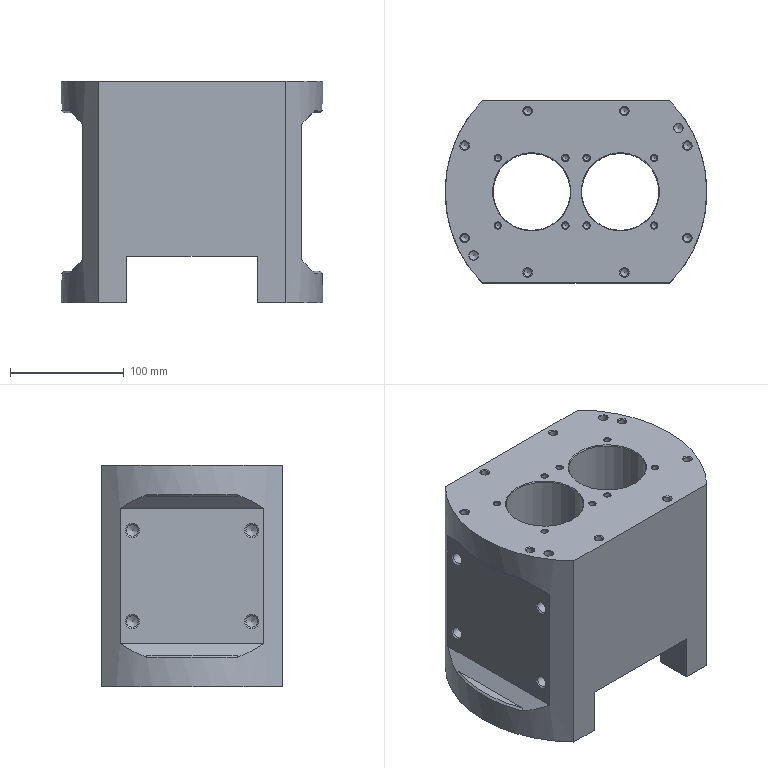NC program | NX | posted with a generic post | part box 230 x 160 x 195 mm
Lines 2916 to 3764 of 6533:
(ZLEVEL_PROFILE_COPY_1 , TOOL : D6R0.5)
N5818 T05 M6
N5820 G54
N5822 G17 G0 G90 X68.093 Y-13.204 B0. C0. S6500 M3
N5824 G43 Z30. H5
N5826 Z2.929
N5828 G94 G1 Z-0.071 F1000.
N5830 X68.902 Y-12.62
N5832 G3 X69.147 Y-12.072 R0.6
N5834 G2 X69.147 Y12.07 R118.03 F2500.
N5836 G1 X69.145 Y12.24 Z-0.088
N5838 X69.146 Y12.409 Z-0.106
N5840 X69.147 Y12.577 Z-0.124
N5842 X69.149 Y12.746 Z-0.141
N5844 G3 X69.149 Y-12.747 R117.508
N5846 G1 X69.148 Y-12.91 Z-0.159
N5848 X69.149 Y-13.072 Z-0.177
N5850 Y-13.235 Z-0.194
N5852 X69.151 Y-13.397 Z-0.212
N5854 G2 X69.151 Y13.397 R117.429
N5856 G1 X69.149 Y13.555 Z-0.23
N5858 Y13.713 Z-0.247
N5860 Y13.871 Z-0.265
N5862 X69.153 Y14.029 Z-0.283
N5864 G3 X69.153 Y-14.027 R117.401
N5866 G1 X69.151 Y-14.173 Z-0.301
N5868 Y-14.319 Z-0.318
N5870 X69.152 Y-14.465 Z-0.336
N5872 X69.154 Y-14.611 Z-0.354
N5874 G2 X69.154 Y14.61 R117.367
N5876 G1 X69.153 Y14.756 Z-0.371
N5878 Y14.902 Z-0.389
N5880 Y15.047 Z-0.407
N5882 X69.155 Y15.193 Z-0.424
N5884 G3 X69.154 Y-15.192 R117.732
N5886 G1 X69.153 Y-15.327 Z-0.442
N5888 X69.154 Y-15.461 Z-0.46
N5890 Y-15.596 Z-0.477
N5892 X69.157 Y-15.73 Z-0.495
N5894 G2 X69.157 Y15.731 R117.468
N5896 G1 X69.156 Y15.862 Z-0.513
N5898 Y15.994 Z-0.53
N5900 Y16.125 Z-0.548
N5902 X69.157 Y16.256 Z-0.566
N5904 G3 X69.157 Y-16.255 R117.679
N5906 G1 Y-16.387 Z-0.583
N5908 Y-16.518 Z-0.601
N5910 X69.158 Y-16.649 Z-0.619
N5912 X69.16 Y-16.78 Z-0.636
N5914 G2 X69.16 Y16.781 R117.696
N5916 G1 X69.157 Y16.946 Z-0.66
N5918 X69.158 Y17.111 Z-0.684
N5920 X69.16 Y17.275 Z-0.707
N5922 G3 X69.16 Y-17.276 R117.851
N5924 G1 Y-17.436 Z-0.731
N5926 X69.161 Y-17.595 Z-0.754
N5928 X69.163 Y-17.755 Z-0.778
N5930 G2 X69.163 Y17.755 R117.722
N5932 G1 X69.162 Y17.914 Z-0.801
N5934 Y18.074 Z-0.825
N5936 X69.165 Y18.233 Z-0.849
N5938 G3 X69.165 Y-18.234 R117.882
N5940 G1 X69.162 Y-18.385 Z-0.872
N5942 X69.163 Y-18.535 Z-0.896
N5944 X69.164 Y-18.684 Z-0.919
N5946 G2 X69.164 Y18.683 R117.992
N5948 G1 X69.165 Y18.83 Z-0.943
N5950 Y18.978 Z-0.966
N5952 X69.169 Y19.124 Z-0.99
N5954 G3 X69.169 Y-19.124 R117.692
N5956 G1 X69.166 Y-19.271 Z-1.014
N5958 X69.167 Y-19.418 Z-1.037
N5960 X69.171 Y-19.564 Z-1.061
N5962 G2 X69.171 Y19.564 R117.719
N5964 G1 X69.167 Y19.71 Z-1.084
N5966 Y19.855 Z-1.108
N5968 X69.171 Y20. Z-1.131
N5970 G3 X69.171 Y-19.999 R117.986
N5972 G1 X69.169 Y-20.137 Z-1.155
N5974 Y-20.274 Z-1.179
N5976 X69.17 Y-20.411 Z-1.202
N5978 G2 X69.17 Y20.411 R118.312
N5980 G1 Y20.547 Z-1.226
N5982 X69.171 Y20.682 Z-1.249
N5984 X69.173 Y20.817 Z-1.273
N5986 G3 X69.173 Y-20.817 R118.165
N5988 G1 X69.172 Y-20.953 Z-1.296
N5990 Y-21.088 Z-1.32
N5992 X69.176 Y-21.223 Z-1.344
N5994 G2 X69.176 Y21.222 R118.139
N5996 G1 X69.172 Y21.353 Z-1.367
N5998 X69.173 Y21.484 Z-1.391
N6000 X69.178 Y21.613 Z-1.414
N6002 G3 X69.178 Y-21.614 R118.128
N6004 G1 X69.175 Y-21.741 Z-1.438
N6006 Y-21.867 Z-1.461
N6008 X69.18 Y-21.992 Z-1.485
N6010 G2 X69.18 Y21.992 R118.072
N6012 G1 X69.176 Y22.119 Z-1.508
N6014 X69.177 Y22.245 Z-1.532
N6016 X69.181 Y22.37 Z-1.556
N6018 G3 X69.181 Y-22.37 R118.117
N6020 G1 X69.178 Y-22.497 Z-1.579
N6022 Y-22.623 Z-1.603
N6024 X69.182 Y-22.749 Z-1.626
N6026 G2 X69.182 Y22.749 R118.257
N6028 G1 X69.178 Y22.873 Z-1.65
N6030 Y22.996 Z-1.673
N6032 X69.182 Y23.118 Z-1.697
N6034 G3 X69.183 Y-23.118 R118.397
N6036 G1 X69.18 Y-23.237 Z-1.721
N6038 X69.181 Y-23.356 Z-1.744
N6040 X69.184 Y-23.474 Z-1.768
N6042 G2 X69.184 Y23.475 R118.441
N6044 G1 X69.182 Y23.593 Z-1.791
N6046 Y23.711 Z-1.815
N6048 X69.185 Y23.828 Z-1.839
N6050 G3 X69.185 Y-23.828 R118.406
N6052 G1 X69.183 Y-23.947 Z-1.862
N6054 X69.184 Y-24.065 Z-1.886
N6056 X69.186 Y-24.182 Z-1.909
N6058 G2 X69.186 Y24.181 R118.646
N6060 G1 X69.184 Y24.353 Z-1.945
N6062 X69.187 Y24.525 Z-1.98
N6064 G3 X69.187 Y-24.526 R118.613
N6066 G1 X69.186 Y-24.693 Z-2.016
N6068 X69.189 Y-24.858 Z-2.051
N6070 G2 X66.596 Y-3.188 R119.31
N6072 X66.596 Y3.188 R183.596
N6074 X69.189 Y24.859 R119.287
N6076 G1 X69.188 Y25.025 Z-2.087
N6078 X69.191 Y25.191 Z-2.122
N6080 G3 X66.629 Y5.883 R119.525
N6082 X66.629 Y-5.883 R171.965
N6084 X69.191 Y-25.191 R119.526
N6086 G1 X69.189 Y-25.357 Z-2.158
N6088 X69.193 Y-25.522 Z-2.193
N6090 G2 X66.596 Y-6.489 R118.317
N6092 X66.515 Y0. R174.715
N6094 X66.596 Y6.489 R174.715
N6096 X69.193 Y25.523 R118.333
N6098 G1 X69.19 Y25.689 Z-2.229
N6100 X69.194 Y25.855 Z-2.264
N6102 G3 X66.771 Y10.035 R120.12
N6104 G1 X66.712 Y9.343
N6106 G3 X66.527 Y5.191 R58.855
N6108 X66.53 Y-5.506 R519.675
N6110 X66.684 Y-8.997 R52.487
N6112 X69.195 Y-25.854 R120.659
N6114 G1 X69.191 Y-26.016 Z-2.299
N6116 X69.196 Y-26.176 Z-2.335
N6118 G2 X66.596 Y-8.676 R119.483
N6120 X66.5 Y-4.097 R108.834
N6122 G1 Y4.097
N6124 G2 X66.596 Y8.676 R108.836
N6126 X69.196 Y26.177 R119.535
N6128 G1 X69.193 Y26.336 Z-2.371
N6130 X69.198 Y26.492 Z-2.406
N6132 G3 X66.596 Y9.537 R118.228
N6134 X66.5 Y5.801 R72.503
N6136 G1 Y-5.801
N6138 G3 X66.596 Y-9.537 R72.503
N6140 X69.198 Y-26.492 R118.211
N6142 G1 X69.195 Y-26.649 Z-2.442
N6144 X69.199 Y-26.805 Z-2.477
N6146 G2 X66.717 Y-11.743 R121.153
N6148 X66.52 Y-8.197 R39.615
N6150 G1 X66.5 Y-6.337
N6152 Y7.031
N6154 G2 X66.596 Y10.319 R56.155
N6156 X67.909 Y20.417 R109.838
N6158 X69.199 Y26.805 R114.904
N6160 G1 X69.196 Y26.963 Z-2.513
N6162 X69.2 Y27.118 Z-2.548
N6164 G3 X66.596 Y11.101 R118.148
N6166 X66.5 Y7.493 R60.73
N6168 G1 Y-7.492
N6170 G3 X66.596 Y-11.101 R60.738
N6172 X69.2 Y-27.119 R118.21
N6174 G1 X69.197 Y-27.275 Z-2.584
N6176 X69.201 Y-27.429 Z-2.619
N6178 G2 X66.596 Y-11.868 R120.019
N6180 X66.5 Y-8.498 R55.778
N6182 G1 Y8.502
N6184 G2 X66.596 Y11.868 R55.751
N6186 X69.201 Y27.427 R119.955
N6188 G1 X69.199 Y27.577 Z-2.655
N6190 X69.201 Y27.726 Z-2.691
N6192 G3 X66.596 Y12.501 R118.185
N6194 X66.5 Y9.343 R44.574
N6196 G1 Y-9.343
N6198 G3 X66.596 Y-12.501 R44.574
N6200 X69.201 Y-27.727 R118.22
N6202 G1 X69.2 Y-27.876 Z-2.726
N6204 X69.201 Y-28.024 Z-2.762
N6206 G2 X66.772 Y-14.747 R124.986
N6208 X66.5 Y-10.475 R33.732
N6210 G1 Y10.475
N6212 G2 X66.772 Y14.747 R33.735
N6214 X69.201 Y28.023 R124.948
N6216 G1 X69.202 Y28.172 Z-2.798
N6218 X69.204 Y28.319 Z-2.833
N6220 G3 X66.722 Y14.88 R122.645
N6222 X66.5 Y10.976 R30.452
N6224 G1 Y-10.98
N6226 G3 X66.764 Y-15.226 R30.621
N6228 G1 X66.813 Y-15.572
N6230 G3 X69.204 Y-28.32 R122.05
N6232 G1 X69.203 Y-28.468 Z-2.869
N6234 X69.207 Y-28.615 Z-2.905
N6236 G2 X66.596 Y-14.327 R118.038
N6238 X66.5 Y-11.69 R36.45
N6240 G1 Y11.685
N6242 G2 X66.596 Y14.327 R36.451
N6244 X69.207 Y28.616 R118.098
N6246 G1 X69.204 Y28.765 Z-2.94
N6248 X69.209 Y28.913 Z-2.976
N6250 G3 X66.596 Y14.925 R120.144
N6252 X66.5 Y12.357 R35.663
N6254 G1 Y-12.353
N6256 G3 X66.596 Y-14.925 R35.662
N6258 X69.209 Y-28.912 R119.707
N6260 G1 X69.205 Y-29.057 Z-3.012
N6262 X69.21 Y-29.201 Z-3.047
N6264 G2 X66.596 Y-15.424 R117.666
N6266 X66.5 Y-12.987 R29.137
N6268 G1 Y12.989
N6270 G2 X66.596 Y15.424 R29.129
N6272 X69.21 Y29.202 R117.732
N6274 G1 X69.207 Y29.343 Z-3.083
N6276 X69.21 Y29.483 Z-3.119
N6278 G3 X66.776 Y17.302 R123.214
N6280 G1 X66.73 Y16.956
N6282 X66.596 Y15.922
N6284 G3 X66.5 Y13.59 R26.367
N6286 G1 Y-13.597
N6288 G3 X66.596 Y-15.922 R26.354
N6290 G1 X66.73 Y-16.956
N6292 X66.776 Y-17.302
N6294 G3 X69.21 Y-29.482 R123.08
N6296 G1 X69.208 Y-29.624 Z-3.155
N6298 X69.209 Y-29.765 Z-3.191
N6300 G2 X66.756 Y-17.648 R125.317
N6302 X66.5 Y-14.169 R21.723
N6304 G1 Y14.174
N6306 G2 X66.756 Y17.648 R21.71
N6308 X69.209 Y29.765 R125.299
N6310 G1 X69.21 Y29.905 Z-3.226
N6312 X69.212 Y30.045 Z-3.262
N6314 G3 X66.737 Y17.994 R125.463
N6316 X66.5 Y14.725 R20.848
N6318 G1 Y-14.727
N6320 G3 X66.737 Y-17.994 R20.845
N6322 X69.212 Y-30.047 R125.682
N6324 G1 X69.211 Y-30.187 Z-3.298
N6326 X69.215 Y-30.325 Z-3.334
N6328 G2 X66.626 Y-17.648 R120.218
N6330 X66.5 Y-15.226 R21.31
N6332 G1 Y15.226
N6334 X66.503 Y15.572
N6336 G2 X66.725 Y18.34 R17.715
N6338 X69.215 Y30.324 R116.852
N6340 G1 X69.212 Y30.462 Z-3.37
N6342 X69.216 Y30.597 Z-3.405
N6344 G3 X66.61 Y17.994 R119.169
N6346 X66.5 Y15.78 R21.929
N6348 G1 Y-15.778
N6350 G3 X66.61 Y-17.994 R21.933
N6352 X69.216 Y-30.597 R119.73
N6354 G1 X69.214 Y-30.732 Z-3.441
N6356 X69.217 Y-30.865 Z-3.477
N6358 G2 X66.755 Y-19.379 R121.808
N6360 G1 X66.596 Y-18.326
N6362 G2 X66.5 Y-16.264 R20.859
N6364 G1 Y16.264
N6366 G2 X66.596 Y18.326 R20.859
N6368 G1 X66.755 Y19.379
N6370 G2 X69.217 Y30.865 R121.735
N6372 G1 X69.215 Y31. Z-3.513
N6374 X69.216 Y31.134 Z-3.549
N6376 G3 X66.798 Y20.071 R124.289
N6378 G1 X66.743 Y19.725
N6380 X66.596 Y18.748
N6382 G3 X66.5 Y16.768 R20.093
N6384 G1 Y-16.764
N6386 G3 X66.596 Y-18.748 R20.099
N6388 G1 X66.743 Y-19.725
N6390 X66.798 Y-20.071
N6392 G3 X69.216 Y-31.134 R124.191
N6394 G1 X69.217 Y-31.268 Z-3.585
N6396 X69.22 Y-31.401 Z-3.621
N6398 G2 X66.786 Y-20.417 R124.511
N6400 G1 X66.732 Y-20.071
N6402 X66.596 Y-19.17
N6404 G2 X66.5 Y-17.24 R19.316
N6406 G1 Y17.236
N6408 G2 X66.596 Y19.17 R19.32
N6410 G1 X66.732 Y20.071
N6412 X66.786 Y20.417
N6414 G2 X69.22 Y31.402 R124.586
N6416 G1 X69.218 Y31.536 Z-3.656
N6418 X69.222 Y31.67 Z-3.692
N6420 G3 X66.773 Y20.763 R126.599
N6422 X66.5 Y17.7 R16.386
N6424 G1 Y-17.696
N6426 G3 X66.773 Y-20.763 R16.389
N6428 X69.222 Y-31.669 R126.445
N6430 G1 X69.219 Y-31.803 Z-3.728
N6432 X69.223 Y-31.935 Z-3.764
N6434 G2 X66.765 Y-21.109 R127.951
N6436 X66.5 Y-18.147 R15.938
N6438 G1 Y18.144
N6440 G2 X66.765 Y21.109 R15.942
N6442 X69.222 Y31.936 R128.169
N6444 G1 X69.22 Y32.068 Z-3.8
N6446 X69.222 Y32.198 Z-3.836
N6448 G3 X66.766 Y21.524 R131.861
N6450 X66.5 Y18.585 R15.687
N6452 G1 Y-18.582
N6454 G3 X66.695 Y-21.109 R15.69
N6456 X69.222 Y-32.198 R129.86
N6458 G1 Y-32.326 Z-3.872
N6460 X69.225 Y-32.453 Z-3.908
N6462 G2 X66.692 Y-21.463 R126.007
N6464 X66.528 Y-19.915 R10.297
N6466 G1 X66.5 Y-19.011
N6468 Y19.009
N6470 G2 X66.596 Y20.847 R18.921
N6472 X67.304 Y24.569 R68.628
N6474 G1 X67.553 Y25.713
N6476 G2 X69.225 Y32.454 R119.667
N6478 G1 X69.223 Y32.582 Z-3.944
N6480 X69.227 Y32.709 Z-3.98
N6482 G3 X66.742 Y22.113 R125.211
N6484 X66.5 Y19.429 R13.936
N6486 G1 Y-19.427
N6488 G3 X66.687 Y-21.801 R13.941
N6490 X69.227 Y-32.709 R124.165
N6492 G1 X69.225 Y-32.838 Z-4.016
N6494 X69.228 Y-32.965 Z-4.052
N6496 G2 X66.683 Y-22.147 R124.5
N6498 X66.5 Y-19.837 R13.308
N6500 G1 Y19.836
N6502 G2 X66.738 Y22.452 R13.312
N6504 X69.228 Y32.965 R125.755
N6506 G1 X69.226 Y33.093 Z-4.088
N6508 X69.227 Y33.221 Z-4.124
N6510 G3 X66.746 Y22.839 R127.156
N6512 X66.5 Y20.238 R12.858
N6514 G1 Y-20.237
N6516 G3 X66.746 Y-22.839 R12.86
N6518 X69.227 Y-33.222 R127.385
N6520 G1 X69.226 Y-33.346 Z-4.16
N6522 X69.23 Y-33.469 Z-4.196
N6524 G2 X66.758 Y-23.283 R128.86
N6526 X66.5 Y-20.673 R13.313
N6528 G1 Y20.672
N6530 G2 X66.758 Y23.282 R13.316
N6532 X69.23 Y33.468 R128.524
N6534 G1 X69.229 Y33.592 Z-4.232
N6536 X69.232 Y33.714 Z-4.269
N6538 G3 X66.738 Y23.531 R127.393
N6540 X66.5 Y21.016 R12.713
N6542 G1 Y-21.017
N6544 G3 X66.738 Y-23.531 R12.711
N6546 X69.232 Y-33.714 R127.608
N6548 G1 X69.23 Y-33.837 Z-4.305
N6550 X69.232 Y-33.959 Z-4.341
N6552 G2 X66.756 Y-23.968 R129.142
N6554 X66.5 Y-21.456 R12.455
N6556 G1 Y21.455
N6558 G2 X66.756 Y23.968 R12.459
N6560 X69.232 Y33.959 R129.042
N6562 G1 Y34.082 Z-4.377
N6564 X69.234 Y34.204 Z-4.413
N6566 G3 X66.785 Y24.5 R134.606
N6568 X66.5 Y21.766 R12.991
N6570 G1 Y-21.769
N6572 G3 X66.668 Y-23.877 R12.956
N6574 X69.234 Y-34.203 R128.002
N6576 G1 X69.233 Y-34.326 Z-4.449
N6578 X69.236 Y-34.447 Z-4.485
N6580 G2 X66.672 Y-24.223 R125.671
N6582 X66.5 Y-22.132 R11.933
N6584 G1 Y22.136
N6586 G2 X66.76 Y24.68 R11.926
N6588 X69.236 Y34.448 R129.138
N6590 G1 X69.234 Y34.572 Z-4.522
N6592 X69.237 Y34.694 Z-4.558
N6594 G3 X66.75 Y24.945 R128.587
N6596 X66.5 Y22.492 R11.31
N6598 G1 Y-22.493
N6600 G3 X66.676 Y-24.569 R11.314
N6602 X69.237 Y-34.692 R125.279
N6604 G1 X69.236 Y-34.816 Z-4.594
N6606 X69.237 Y-34.938 Z-4.63
N6608 G2 X66.728 Y-25.142 R127.473
N6610 X66.5 Y-22.987 R10.291
N6612 G1 Y22.987
N6614 G2 X66.728 Y25.143 R10.29
N6616 X69.236 Y34.939 R127.927
N6618 G1 Y35.057 Z-4.666
N6620 X69.24 Y35.174 Z-4.702
N6622 G3 X66.733 Y25.489 R126.082
N6624 X66.5 Y23.312 R10.273
N6626 G1 Y-23.311
N6628 G3 X66.733 Y-25.489 R10.278
N6630 X69.24 Y-35.173 R125.853
N6632 G1 X69.238 Y-35.292 Z-4.739
N6634 X69.241 Y-35.409 Z-4.775
N6636 G2 X66.764 Y-25.954 R126.985
N6638 X66.5 Y-23.531 R10.617
N6640 G1 Y23.531
N6642 G2 X66.764 Y25.954 R10.617
N6644 X69.241 Y35.41 R127.154
N6646 G1 X69.24 Y35.528 Z-4.811
N6648 X69.241 Y35.645 Z-4.847
N6650 G3 X66.768 Y26.3 R131.551
N6652 X66.5 Y23.877 R10.618
N6654 G1 Y-23.877
N6656 G3 X66.768 Y-26.3 R10.618
N6658 X69.24 Y-35.644 R131.588
N6660 G1 X69.241 Y-35.762 Z-4.884
N6662 X69.244 Y-35.878 Z-4.92
N6664 G2 X66.773 Y-26.646 R133.034
N6666 X66.5 Y-24.213 R10.585
N6668 G1 Y24.212
N6670 G2 X66.773 Y26.646 R10.587
N6672 X69.244 Y35.879 R132.823
N6674 G1 X69.243 Y35.996 Z-4.956
N6676 X69.246 Y36.112 Z-4.993
N6678 G3 X66.778 Y26.991 R135.109
N6680 X66.5 Y24.541 R10.624
N6682 G1 Y-24.543
N6684 G3 X66.703 Y-26.646 R10.616
N6686 X69.245 Y-36.112 R132.809
N6688 G1 X69.243 Y-36.23 Z-5.029
N6690 X69.245 Y-36.346 Z-5.065
N6692 G2 X66.645 Y-26.646 R119.234
N6694 X66.5 Y-24.866 R10.596
N6696 G1 Y24.87
N6698 G2 X66.772 Y27.254 R10.218
N6700 X69.245 Y36.345 R136.535
N6702 G1 X69.246 Y36.458 Z-5.102
N6704 X69.249 Y36.57 Z-5.138
N6706 G3 X66.788 Y27.591 R127.352
N6708 X66.596 Y26.669 R18.236
N6710 X66.5 Y25.187 R12.084
N6712 G1 Y-25.189
N6714 X66.52 Y-25.797
N6716 G3 X66.719 Y-27.304 R7.766
N6718 X69.248 Y-36.57 R129.218
N6720 G1 X69.247 Y-36.684 Z-5.174
N6722 X69.25 Y-36.796 Z-5.211
N6724 G2 X66.824 Y-28.03 R125.907
N6726 G1 X66.74 Y-27.684
N6728 G2 X66.501 Y-25.607 R9.104
N6730 G1 X66.5 Y-25.505
N6732 Y25.504
N6734 X66.501 Y25.607
N6736 G2 X66.74 Y27.684 R9.104
N6738 G1 X66.824 Y28.03
N6740 G2 X69.25 Y36.796 R125.772
N6742 G1 X69.249 Y36.909 Z-5.247
N6744 X69.25 Y37.022 Z-5.283
N6746 G3 X66.754 Y28.03 R127.785
N6748 X66.5 Y25.819 R9.067
N6750 G1 Y-25.816
N6752 G3 X66.754 Y-28.03 R9.072
N6754 X69.25 Y-37.022 R127.765
N6756 G1 Y-37.135 Z-5.32
N6758 X69.253 Y-37.247 Z-5.356
N6760 G2 X66.745 Y-28.28 R124.349
N6762 X66.5 Y-26.208 R8.89
N6764 G1 Y26.209
N6766 G2 X66.745 Y28.279 R8.881
N6768 X69.253 Y37.247 R124.438
N6770 G1 X69.252 Y37.361 Z-5.393
N6772 X69.254 Y37.473 Z-5.429
N6774 G3 X66.781 Y28.722 R127.03
N6776 X66.5 Y26.431 R9.077
N6778 G1 Y-26.432
N6780 G3 X66.781 Y-28.722 R9.074
N6782 X69.255 Y-37.473 R126.767
N6784 G1 X69.254 Y-37.586 Z-5.466
N6786 X69.255 Y-37.699 Z-5.502
N6788 G2 X66.794 Y-29.068 R131.371
N6790 X66.5 Y-26.732 R9.121
N6792 G1 Y26.736
N6794 G2 X66.794 Y29.068 R9.119
N6796 X69.254 Y37.7 R132.684
N6798 G1 Y37.812 Z-5.538
N6800 X69.258 Y37.923 Z-5.575
N6802 G3 X66.808 Y29.414 R134.287
N6804 X66.5 Y27.031 R9.159
N6806 G1 Y-27.033
N6808 G3 X66.808 Y-29.414 R9.157
N6810 X69.258 Y-37.922 R133.655
N6812 G1 X69.256 Y-38.033 Z-5.611
N6814 X69.259 Y-38.143 Z-5.648
N6816 G2 X66.738 Y-29.414 R134.13
N6818 X66.5 Y-27.327 R8.918
N6820 G1 Y27.327
N6822 G2 X66.774 Y29.559 R8.919
N6824 X69.259 Y38.144 R134.199
N6826 G1 X69.258 Y38.254 Z-5.684
N6828 X69.26 Y38.363 Z-5.721
N6830 G3 X67.093 Y31.042 R132.697
N6832 G1 X66.753 Y29.76
N6834 G3 X66.5 Y27.621 R8.92
N6836 G1 Y-27.618
N6838 G3 X66.753 Y-29.76 R8.922
N6840 G1 X66.844 Y-30.106
N6842 G3 X69.26 Y-38.362 R135.361
N6844 G1 Y-38.471 Z-5.757
N6846 X69.263 Y-38.579 Z-5.794
N6848 G2 X66.686 Y-29.76 R134.37
N6850 X66.5 Y-27.909 R9.207
N6852 G1 Y27.907
N6854 G2 X66.686 Y29.76 R9.171
N6856 X69.263 Y38.581 R135.25
N6858 G1 X69.261 Y38.691 Z-5.83
N6860 X69.263 Y38.8 Z-5.867
N6862 G3 X66.771 Y30.37 R138.332
N6864 X66.5 Y28.193 R8.362
N6866 G1 Y-28.195
N6868 G3 X66.707 Y-30.106 R8.36
N6870 X69.264 Y-38.798 R133.897
N6872 G1 Y-38.908 Z-5.904
N6874 X69.266 Y-39.017 Z-5.94
N6876 G2 X66.754 Y-30.548 R131.862
N6878 X66.5 Y-28.566 R7.861
N6880 G1 Y28.561
N6882 G2 X66.756 Y30.557 R7.906
N6884 X69.266 Y39.019 R133.4
N6886 G1 X69.264 Y39.128 Z-5.977
N6888 X69.267 Y39.236 Z-6.013
N6890 G3 X66.75 Y30.798 R134.266
N6892 X66.5 Y28.757 R7.828
N6894 G1 Y-28.758
N6896 G3 X66.75 Y-30.798 R7.825
N6898 X69.268 Y-39.233 R132.407
N6900 G1 X69.266 Y-39.342 Z-6.05
N6902 X69.267 Y-39.45 Z-6.087
N6904 G2 X66.772 Y-31.144 R136.917
N6906 X66.5 Y-29.035 R7.861
N6908 G1 Y29.033
N6910 G2 X66.772 Y31.144 R7.863
N6912 X69.265 Y39.454 R140.478
N6914 G1 Y39.562 Z-6.123
N6916 X69.268 Y39.67 Z-6.16
N6918 G3 X66.794 Y31.49 R141.118
N6920 X66.5 Y29.311 R7.95
N6922 G1 Y-29.308
N6924 G3 X66.794 Y-31.49 R7.95
N6926 X69.27 Y-39.664 R136.334
N6928 G1 X69.268 Y-39.772 Z-6.197
N6930 X69.27 Y-39.879 Z-6.233
N6932 G2 X66.816 Y-31.836 R143.021
N6934 X66.5 Y-29.582 R8.018
N6936 G1 Y29.581
N6938 G2 X66.816 Y31.836 R8.011
N6940 X69.268 Y39.887 R148.926
N6942 G1 X69.266 Y39.996 Z-6.27
N6944 X69.268 Y40.105 Z-6.307
N6946 G3 X66.792 Y32.016 R162.117
N6948 X66.5 Y29.872 R8.012
N6950 G1 Y-29.87
N6952 G3 X66.79 Y-32.006 R8.02
N6954 X69.271 Y-40.095 R150.851
N6956 G1 X69.27 Y-40.203 Z-6.343
N6958 X69.273 Y-40.31 Z-6.38
N6960 G2 X66.804 Y-32.327 R160.1
N6962 X66.5 Y-30.121 R8.157
N6964 G1 Y30.129
N6966 G2 X66.805 Y32.331 R8.106
N6968 X69.27 Y40.321 R173.434
N6970 G1 X69.263 Y40.419 Z-6.417
N6972 X69.261 Y40.516 Z-6.453
N6974 X68.921 Y39.449
N6976 X68.691 Y38.757
N6978 G3 X66.79 Y32.528 R148.918
N6980 X66.5 Y30.384 R7.94
N6982 G1 Y-30.383
N6984 G3 X66.79 Y-32.528 R7.927
N6986 X69.265 Y-40.503 R169.309
N6988 G1 X69.223 Y-40.594 Z-6.527
N6990 G2 X66.819 Y-32.874 R175.999
N6992 X66.5 Y-30.647 R7.642
N6994 G1 Y30.645
N6996 G2 X66.79 Y32.789 R7.904
N6998 X67.976 Y36.741 R104.768
N7000 G1 X69.228 Y40.635
N7002 X69.185 Y40.758 Z-6.6
N7004 X69.16 Y40.63
N7006 X68.896 Y39.795
N7008 X68.448 Y38.435
N7010 G3 X66.768 Y32.932 R130.952
N7012 X66.5 Y30.99 R7.169
N7014 G1 Y-30.99
N7016 G3 X66.772 Y-32.948 R7.171
N7018 X68.992 Y-40.088 R150.629
N7020 G2 X69.168 Y-40.691 R7.405
N7022 G1 X69.098 Y-40.791 Z-6.674
N7024 G3 X69.007 Y-40.35 R1.813
N7026 G2 X66.685 Y-32.874 R151.323
N7028 X66.5 Y-31.144 R7.693
N7030 G1 Y31.144
N7032 G2 X66.801 Y33.327 R7.693
N7034 X68.953 Y40.162 R147.219
N7036 G3 X69.104 Y40.822 R3.258
N7038 G1 X69.028 Y40.907 Z-6.746
N7040 G2 X68.915 Y40.263 R2.116
N7042 G3 X66.812 Y33.567 R145.846
N7044 X66.5 Y31.416 R7.162
N7046 G1 Y-31.418
N7048 G3 X66.812 Y-33.567 R7.159
N7050 X68.914 Y-40.273 R153.461
N7052 G2 X69.026 Y-40.909 R2.121
N7054 G1 X68.955 Y-41.041 Z-6.819
N7056 X68.912 Y-40.487
N7058 G2 X66.777 Y-33.681 R169.842
N7060 X66.5 Y-31.734 R6.976
N7062 G1 Y31.731
N7064 G2 X66.768 Y33.645 R6.968
N7066 X68.46 Y39.103 R128.924
N7068 G1 X68.647 Y39.657
N7070 X68.914 Y40.487
N7072 X68.957 Y41.039
N7074 X68.881 Y41.17 Z-6.891
N7076 X68.846 Y40.487
N7078 X68.647 Y39.857
N7080 G3 X66.776 Y33.913 R128.398
N7082 X66.5 Y31.911 R6.948
N7084 G1 Y-31.91
N7086 G3 X66.776 Y-33.913 R6.949
N7088 X68.845 Y-40.487 R169.118
N7090 G1 X68.878 Y-41.173
N7092 X68.813 Y-41.298 Z-6.962
N7094 X68.778 Y-40.487
N7096 G2 X66.809 Y-34.259 R172.111
N7098 X66.5 Y-32.153 R7.113
N7100 G1 Y32.154
N7102 G2 X66.809 Y34.259 R7.113
N7104 X68.739 Y40.326 R132.303
N7106 G3 X68.786 Y40.576 R0.883
N7108 G1 X68.817 Y41.294
N7110 X68.748 Y41.419 Z-7.033
N7112 X68.715 Y40.547
N7114 G2 X68.675 Y40.335 R0.736
N7116 G3 X66.785 Y34.409 R132.873
N7118 X66.5 Y32.425 R7.049
N7120 G1 Y-32.422
N7122 G3 X66.795 Y-34.447 R7.084
N7124 X68.711 Y-40.487 R183.193
N7126 G1 X68.743 Y-41.423
N7128 X68.67 Y-41.55 Z-7.105
N7130 X68.668 Y-41.526
N7132 X68.644 Y-40.487
N7134 G2 X66.775 Y-34.605 R183.683
N7136 X66.5 Y-32.63 R6.936
N7138 G1 Y32.63
N7140 G2 X66.775 Y34.605 R6.936
N7142 G1 X66.977 Y35.297
N7144 X68.073 Y38.757
N7146 X68.551 Y40.174
N7148 G3 X68.644 Y40.487 R4.248
N7150 G1 X68.675 Y41.545
N7152 X68.61 Y41.687 Z-7.176
N7154 X68.604 Y41.526
N7156 X68.578 Y40.603
N7158 X68.579 Y40.487
N7160 G3 X66.831 Y35.046 R318.592
N7162 X66.5 Y32.867 R7.331
N7164 G1 Y-32.87
N7166 G3 X66.821 Y-35.008 R7.289
N7168 X68.58 Y-40.487 R220.771
N7170 G1 X68.599 Y-41.526
N7172 X68.605 Y-41.694
N7174 X68.535 Y-41.842 Z-7.247
N7176 X68.516 Y-40.487
N7178 G2 X66.842 Y-35.297 R202.898
N7180 X66.5 Y-33.1 R7.165
N7182 G1 Y33.099
N7184 G2 X66.842 Y35.297 R7.165
N7186 X68.515 Y40.487 R207.564
N7188 G1 X68.51 Y40.618
N7190 X68.541 Y41.836
N7192 X68.505 Y41.922 Z-7.282
N7194 X68.476 Y42.008 Z-7.317
N7196 X68.47 Y41.872
N7198 X68.443 Y40.632
N7200 X68.45 Y40.487
N7202 G3 X66.815 Y35.433 R206.042
N7204 X66.5 Y33.353 R7.038
N7206 G1 Y-33.353
N7208 G3 X66.813 Y-35.429 R7.033
N7210 X68.452 Y-40.487 R194.761
N7212 G1 X68.469 Y-42.015
N7214 X68.431 Y-42.104 Z-7.353
N7216 X68.397 Y-42.194 Z-7.388
N7218 X68.396 Y-40.645
N7220 X68.388 Y-40.487
N7222 G2 X66.813 Y-35.643 R175.402
N7224 X66.5 Y-33.556 R6.919
N7226 G1 Y33.557
N7228 G2 X66.813 Y35.643 R6.919
N7230 X68.386 Y40.487 R190.626
N7232 G1 X68.376 Y40.647
N7234 X68.402 Y42.188
N7236 X68.365 Y42.278 Z-7.424
N7238 X68.334 Y42.368 Z-7.459
N7240 X68.312 Y40.661
N7242 X68.322 Y40.487
N7244 G3 X66.799 Y35.816 R156.485
N7246 X66.5 Y33.786 R6.723
N7248 G1 Y-33.784
N7250 G3 X66.748 Y-35.643 R6.724
N7252 X68.324 Y-40.487 R151.59
N7254 G1 X68.331 Y-40.66
N7256 Y-42.373
N7258 X68.293 Y-42.462 Z-7.494
N7260 X68.258 Y-42.551 Z-7.53
N7262 X68.259 Y-40.487
N7264 G2 X66.789 Y-35.989 R143.168
N7266 X66.5 Y-34.011 R6.445
N7268 G1 Y34.009
N7270 G2 X66.789 Y35.989 R6.447
N7272 X68.257 Y40.487 R150.171
N7274 G1 X68.245 Y40.834
N7276 X68.261 Y42.548
N7278 X68.226 Y42.638 Z-7.565
N7280 X68.195 Y42.728 Z-7.6
N7282 X68.19 Y42.564
N7284 X68.181 Y40.834
N7286 X68.193 Y40.695
N7288 Y40.487
N7290 G3 X66.727 Y35.989 R115.714
N7292 X66.5 Y34.232 R6.524
N7294 G1 Y-34.233
N7296 G3 X66.727 Y-35.989 R6.523
N7298 G1 X66.832 Y-36.335
N7300 G3 X68.192 Y-40.487 R132.754
N7302 G1 X68.188 Y-42.564
N7304 X68.194 Y-42.73
N7306 X68.155 Y-42.82 Z-7.636
N7308 X68.12 Y-42.91 Z-7.671
N7310 X68.118 Y-42.564
N7312 X68.121 Y-40.917
N7314 X68.122 Y-40.885
N7316 Y-40.483
N7318 G2 X66.765 Y-36.335 R143.305
N7320 X66.5 Y-34.454 R6.371
N7322 G1 Y34.455
N7324 G2 X66.765 Y36.335 R6.371
N7326 X68.122 Y40.483 R143.305
N7328 G1 Y40.88
N7330 X68.116 Y40.924
N7332 X68.121 Y42.907
N7334 X68.086 Y42.995 Z-7.706
N7336 X68.055 Y43.082 Z-7.742
N7338 X68.05 Y42.91
N7340 X68.047 Y41.18
N7342 X68.051 Y40.834
N7344 Y40.47
N7346 G3 X66.808 Y36.681 R135.412
N7348 X66.5 Y34.677 R6.41
N7350 G1 Y-34.676
N7352 G3 X66.808 Y-36.681 R6.411
N7354 X68.051 Y-40.47 R137.079
N7356 G1 Y-41.099
N7358 X68.05 Y-42.91
N7360 X68.054 Y-43.083
N7362 X68.015 Y-43.171 Z-7.777
N7364 X67.979 Y-43.258 Z-7.812
N7366 X67.98 Y-41.284
N7368 Y-40.457
N7370 G2 X66.79 Y-36.833 R131.346
N7372 X66.5 Y-34.933 R6.37
N7374 G1 Y34.933
N7376 G2 X66.79 Y36.833 R6.37
N7378 X67.98 Y40.457 R131.346
N7380 G1 Y41.284
N7382 Y43.257
N7384 X67.945 Y43.345 Z-7.848
N7386 X67.912 Y43.432 Z-7.883
N7388 X67.91 Y41.468
N7390 Y40.444
N7392 G3 X66.784 Y37.027 R129.758
N7394 X66.5 Y35.111 R6.299
N7396 G1 Y-35.111
N7398 G3 X66.784 Y-37.027 R6.299
N7400 X67.91 Y-40.444 R129.758
N7402 G1 Y-41.468
N7404 X67.909 Y-41.526
N7406 Y-43.256
N7408 X67.912 Y-43.433
N7410 X67.874 Y-43.52 Z-7.918
N7412 X67.839 Y-43.607 Z-7.954
N7414 X67.838 Y-41.652
N7416 X67.839 Y-41.526
N7418 Y-40.431
N7420 G2 X66.827 Y-37.373 R131.496
N7422 X66.5 Y-35.327 R6.426
N7424 G1 Y35.328
N7426 G2 X66.827 Y37.373 R6.426
N7428 X67.839 Y40.431 R131.496
N7430 G1 Y41.526
N7432 X67.836 Y41.872
N7434 X67.839 Y43.606
N7436 X67.803 Y43.694 Z-7.989
N7438 X67.774 Y43.781 Z-8.025
N7440 X67.768 Y43.602
N7442 X67.766 Y41.872
N7444 X67.768 Y41.526
N7446 Y40.418
N7448 X66.98 Y38.065
N7450 X66.798 Y37.492
N7452 G3 X66.5 Y35.564 R6.388
N7454 G1 Y-35.564
N7456 G3 X66.798 Y-37.492 R6.388
N7458 G1 X66.98 Y-38.065
N7460 X67.768 Y-40.418
N7462 Y-41.526
N7464 X67.767 Y-41.833
N7466 X67.768 Y-43.602
N7468 X67.774 Y-43.781
N7470 X67.732 Y-43.868 Z-8.06
N7472 X67.698 Y-43.956 Z-8.095
N7474 X67.696 Y-42.014
N7476 X67.698 Y-41.872
N7478 Y-40.405
N7480 X66.913 Y-38.065
N7482 X66.803 Y-37.719
N7484 G2 X66.5 Y-35.756 R6.361
N7486 G1 Y35.755
N7488 G2 X66.803 Y37.719 R6.361
N7490 G1 X66.913 Y38.065
N7492 X67.698 Y40.405
N7494 Y41.872
N7496 X67.696 Y42.014
N7498 X67.698 Y43.956
N7500 X67.662 Y44.043 Z-8.131
N7502 X67.629 Y44.13 Z-8.166
N7504 X67.627 Y43.948
N7506 Y41.872
N7508 X67.626 Y40.382